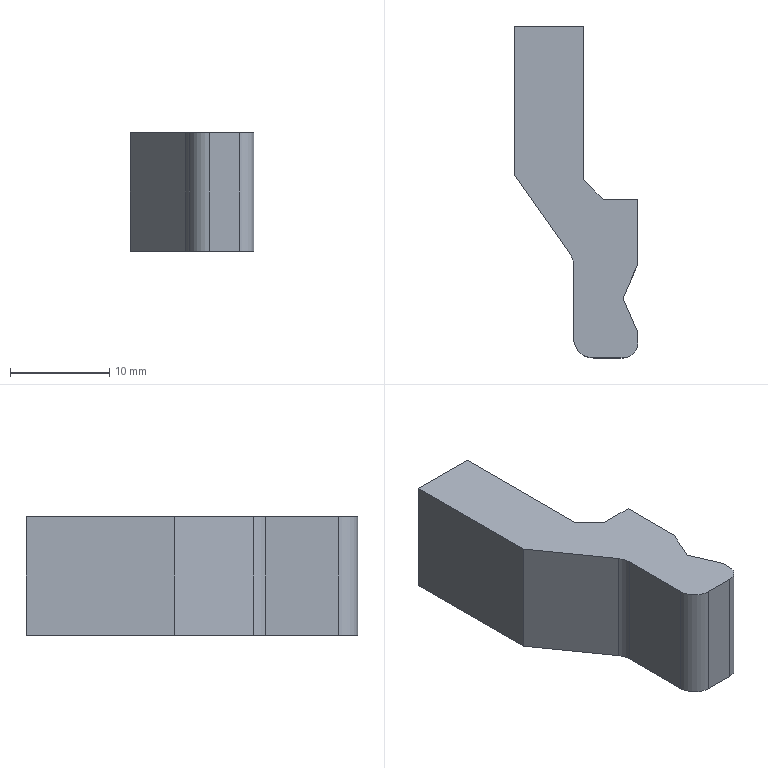Part | STEP file | PN_0018 | 1 solid | 21 faces | box 12.5 x 33.5 x 12 mm | volume 2479 mm3 | plane 18 | cylinder 3 | commonest cylinder face diameters 4 x2 3 x1